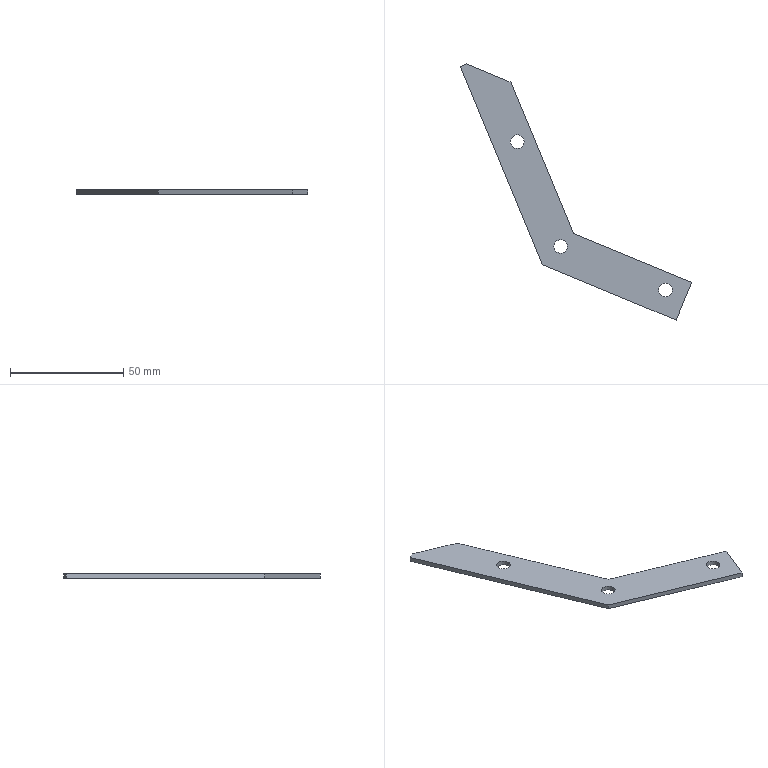Part | SolidWorks | features ICE 6, Cut 1, Extrusion 1, Shell 1 | 1 solid | 15 faces | box 102.016 x 112.94 x 2 mm | volume 5038 mm3 | plane 9 | cylinder 6 | commonest cylinder face diameters 6 x6
STEP:
#1=CARTESIAN_POINT('',(-66.636,-128.964,308.));
#2=VERTEX_POINT('',#1);
#3=CARTESIAN_POINT('',(-60.636,-128.964,308.));
#4=VERTEX_POINT('',#3);
#5=CARTESIAN_POINT('',(-63.636,-128.964,308.));
#6=DIRECTION('',(0.,0.,1.));
#7=DIRECTION('',(1.,0.,0.));
#8=AXIS2_PLACEMENT_3D('',#5,#6,#7);
#9=CIRCLE('',#8,3.);
#10=EDGE_CURVE('',#2,#4,#9,.T.);
#11=ORIENTED_EDGE('',*,*,#10,.F.);
#12=CARTESIAN_POINT('',(-66.636,-128.964,310.));
#13=VERTEX_POINT('',#12);
#14=CARTESIAN_POINT('',(-66.636,-128.964,300.));
#15=DIRECTION('',(0.,0.,1.));
#16=VECTOR('',#15,1000.);
#17=LINE('',#14,#16);
#18=EDGE_CURVE('',#2,#13,#17,.T.);
#19=ORIENTED_EDGE('',*,*,#18,.T.);
#20=CARTESIAN_POINT('',(-60.636,-128.964,310.));
#21=VERTEX_POINT('',#20);
#22=CARTESIAN_POINT('',(-63.636,-128.964,310.));
#23=DIRECTION('',(0.,0.,1.));
#24=DIRECTION('',(-1.,0.,0.));
#25=AXIS2_PLACEMENT_3D('',#22,#23,#24);
#26=CIRCLE('',#25,3.);
#27=EDGE_CURVE('',#13,#21,#26,.T.);
#28=ORIENTED_EDGE('',*,*,#27,.T.);
#29=CARTESIAN_POINT('',(-60.636,-128.964,300.));
#30=DIRECTION('',(0.,0.,1.));
#31=VECTOR('',#30,1000.);
#32=LINE('',#29,#31);
#33=EDGE_CURVE('',#4,#21,#32,.T.);
#34=ORIENTED_EDGE('',*,*,#33,.F.);
#35=EDGE_LOOP('',(#11,#19,#28,#34));
#36=FACE_OUTER_BOUND('',#35,.T.);
#37=CARTESIAN_POINT('',(-63.636,-128.964,300.));
#38=DIRECTION('',(0.,0.,1.));
#39=DIRECTION('',(1.,0.,0.));
#40=AXIS2_PLACEMENT_3D('',#37,#38,#39);
#41=CYLINDRICAL_SURFACE('',#40,3.);
#42=ADVANCED_FACE('',(#36),#41,.F.);
#43=CARTESIAN_POINT('',(-112.83,-109.83,308.));
#44=VERTEX_POINT('',#43);
#45=CARTESIAN_POINT('',(-106.83,-109.83,308.));
#46=VERTEX_POINT('',#45);
#47=CARTESIAN_POINT('',(-109.83,-109.83,308.));
#48=DIRECTION('',(0.,0.,1.));
#49=DIRECTION('',(1.,0.,0.));
#50=AXIS2_PLACEMENT_3D('',#47,#48,#49);
#51=CIRCLE('',#50,3.);
#52=EDGE_CURVE('',#44,#46,#51,.T.);
#53=ORIENTED_EDGE('',*,*,#52,.F.);
#54=CARTESIAN_POINT('',(-112.83,-109.83,310.));
#55=VERTEX_POINT('',#54);
#56=CARTESIAN_POINT('',(-112.83,-109.83,300.));
#57=DIRECTION('',(0.,0.,1.));
#58=VECTOR('',#57,1000.);
#59=LINE('',#56,#58);
#60=EDGE_CURVE('',#44,#55,#59,.T.);
#61=ORIENTED_EDGE('',*,*,#60,.T.);
#62=CARTESIAN_POINT('',(-106.83,-109.83,310.));
#63=VERTEX_POINT('',#62);
#64=CARTESIAN_POINT('',(-109.83,-109.83,310.));
#65=DIRECTION('',(0.,0.,1.));
#66=DIRECTION('',(-1.,0.,0.));
#67=AXIS2_PLACEMENT_3D('',#64,#65,#66);
#68=CIRCLE('',#67,3.);
#69=EDGE_CURVE('',#55,#63,#68,.T.);
#70=ORIENTED_EDGE('',*,*,#69,.T.);
#71=CARTESIAN_POINT('',(-106.83,-109.83,300.));
#72=DIRECTION('',(0.,0.,1.));
#73=VECTOR('',#72,1000.);
#74=LINE('',#71,#73);
#75=EDGE_CURVE('',#46,#63,#74,.T.);
#76=ORIENTED_EDGE('',*,*,#75,.F.);
#77=EDGE_LOOP('',(#53,#61,#70,#76));
#78=FACE_OUTER_BOUND('',#77,.T.);
#79=CARTESIAN_POINT('',(-109.83,-109.83,300.));
#80=DIRECTION('',(0.,0.,1.));
#81=DIRECTION('',(1.,0.,0.));
#82=AXIS2_PLACEMENT_3D('',#79,#80,#81);
#83=CYLINDRICAL_SURFACE('',#82,3.);
#84=ADVANCED_FACE('',(#78),#83,.F.);
#85=CARTESIAN_POINT('',(-131.964,-63.636,308.));
#86=VERTEX_POINT('',#85);
#87=CARTESIAN_POINT('',(-125.964,-63.636,308.));
#88=VERTEX_POINT('',#87);
#89=CARTESIAN_POINT('',(-128.964,-63.636,308.));
#90=DIRECTION('',(0.,0.,1.));
#91=DIRECTION('',(1.,0.,0.));
#92=AXIS2_PLACEMENT_3D('',#89,#90,#91);
#93=CIRCLE('',#92,3.);
#94=EDGE_CURVE('',#86,#88,#93,.T.);
#95=ORIENTED_EDGE('',*,*,#94,.F.);
#96=CARTESIAN_POINT('',(-131.964,-63.636,310.));
#97=VERTEX_POINT('',#96);
#98=CARTESIAN_POINT('',(-131.964,-63.636,300.));
#99=DIRECTION('',(0.,0.,1.));
#100=VECTOR('',#99,1000.);
#101=LINE('',#98,#100);
#102=EDGE_CURVE('',#86,#97,#101,.T.);
#103=ORIENTED_EDGE('',*,*,#102,.T.);
#104=CARTESIAN_POINT('',(-125.964,-63.636,310.));
#105=VERTEX_POINT('',#104);
#106=CARTESIAN_POINT('',(-128.964,-63.636,310.));
#107=DIRECTION('',(0.,0.,1.));
#108=DIRECTION('',(-1.,0.,0.));
#109=AXIS2_PLACEMENT_3D('',#106,#107,#108);
#110=CIRCLE('',#109,3.);
#111=EDGE_CURVE('',#97,#105,#110,.T.);
#112=ORIENTED_EDGE('',*,*,#111,.T.);
#113=CARTESIAN_POINT('',(-125.964,-63.636,300.));
#114=DIRECTION('',(0.,0.,1.));
#115=VECTOR('',#114,1000.);
#116=LINE('',#113,#115);
#117=EDGE_CURVE('',#88,#105,#116,.T.);
#118=ORIENTED_EDGE('',*,*,#117,.F.);
#119=EDGE_LOOP('',(#95,#103,#112,#118));
#120=FACE_OUTER_BOUND('',#119,.T.);
#121=CARTESIAN_POINT('',(-128.964,-63.636,300.));
#122=DIRECTION('',(0.,0.,1.));
#123=DIRECTION('',(1.,0.,0.));
#124=AXIS2_PLACEMENT_3D('',#121,#122,#123);
#125=CYLINDRICAL_SURFACE('',#124,3.);
#126=ADVANCED_FACE('',(#120),#125,.F.);
#127=CARTESIAN_POINT('',(-154.061,-30.485,310.));
#128=VERTEX_POINT('',#127);
#129=CARTESIAN_POINT('',(-151.289,-29.337,310.));
#130=VERTEX_POINT('',#129);
#131=CARTESIAN_POINT('',(-154.061,-30.485,310.));
#132=DIRECTION('',(0.9239,0.3827,0.));
#133=VECTOR('',#132,1000.);
#134=LINE('',#131,#133);
#135=EDGE_CURVE('',#128,#130,#134,.T.);
#136=ORIENTED_EDGE('',*,*,#135,.F.);
#137=CARTESIAN_POINT('',(-117.866,-117.866,310.));
#138=VERTEX_POINT('',#137);
#139=CARTESIAN_POINT('',(-155.209,-27.714,310.));
#140=DIRECTION('',(-0.3827,0.9239,0.));
#141=VECTOR('',#140,1000.);
#142=LINE('',#139,#141);
#143=EDGE_CURVE('',#138,#128,#142,.T.);
#144=ORIENTED_EDGE('',*,*,#143,.F.);
#145=CARTESIAN_POINT('',(-58.933,-142.277,310.));
#146=VERTEX_POINT('',#145);
#147=CARTESIAN_POINT('',(-117.866,-117.866,310.));
#148=DIRECTION('',(-0.9239,0.3827,0.));
#149=VECTOR('',#148,1000.);
#150=LINE('',#147,#149);
#151=EDGE_CURVE('',#146,#138,#150,.T.);
#152=ORIENTED_EDGE('',*,*,#151,.F.);
#153=CARTESIAN_POINT('',(-52.045,-125.648,310.));
#154=VERTEX_POINT('',#153);
#155=CARTESIAN_POINT('',(70.138,169.329,310.));
#156=DIRECTION('',(-0.3827,-0.9239,0.));
#157=VECTOR('',#156,1000.);
#158=LINE('',#155,#157);
#159=EDGE_CURVE('',#154,#146,#158,.T.);
#160=ORIENTED_EDGE('',*,*,#159,.F.);
#161=CARTESIAN_POINT('',(-104.09,-104.09,310.));
#162=VERTEX_POINT('',#161);
#163=CARTESIAN_POINT('',(-104.09,-104.09,310.));
#164=DIRECTION('',(0.9239,-0.3827,0.));
#165=VECTOR('',#164,1000.);
#166=LINE('',#163,#165);
#167=EDGE_CURVE('',#162,#154,#166,.T.);
#168=ORIENTED_EDGE('',*,*,#167,.F.);
#169=CARTESIAN_POINT('',(-131.691,-37.455,310.));
#170=VERTEX_POINT('',#169);
#171=CARTESIAN_POINT('',(-147.205,0.,310.));
#172=DIRECTION('',(0.3827,-0.9239,0.));
#173=VECTOR('',#172,1000.);
#174=LINE('',#171,#173);
#175=EDGE_CURVE('',#170,#162,#174,.T.);
#176=ORIENTED_EDGE('',*,*,#175,.F.);
#177=CARTESIAN_POINT('',(-208.989,-5.437,310.));
#178=DIRECTION('',(0.9239,-0.3827,0.));
#179=VECTOR('',#178,1000.);
#180=LINE('',#177,#179);
#181=EDGE_CURVE('',#130,#170,#180,.T.);
#182=ORIENTED_EDGE('',*,*,#181,.F.);
#183=EDGE_LOOP('',(#136,#144,#152,#160,#168,#176,#182));
#184=FACE_OUTER_BOUND('',#183,.T.);
#185=CARTESIAN_POINT('',(-63.636,-128.964,310.));
#186=DIRECTION('',(0.,0.,1.));
#187=DIRECTION('',(-1.,0.,0.));
#188=AXIS2_PLACEMENT_3D('',#185,#186,#187);
#189=CIRCLE('',#188,3.);
#190=EDGE_CURVE('',#21,#13,#189,.T.);
#191=ORIENTED_EDGE('',*,*,#190,.F.);
#192=ORIENTED_EDGE('',*,*,#27,.F.);
#193=EDGE_LOOP('',(#191,#192));
#194=FACE_BOUND('',#193,.T.);
#195=CARTESIAN_POINT('',(-109.83,-109.83,310.));
#196=DIRECTION('',(0.,0.,1.));
#197=DIRECTION('',(-1.,0.,0.));
#198=AXIS2_PLACEMENT_3D('',#195,#196,#197);
#199=CIRCLE('',#198,3.);
#200=EDGE_CURVE('',#63,#55,#199,.T.);
#201=ORIENTED_EDGE('',*,*,#200,.F.);
#202=ORIENTED_EDGE('',*,*,#69,.F.);
#203=EDGE_LOOP('',(#201,#202));
#204=FACE_BOUND('',#203,.T.);
#205=CARTESIAN_POINT('',(-128.964,-63.636,310.));
#206=DIRECTION('',(0.,0.,1.));
#207=DIRECTION('',(-1.,0.,0.));
#208=AXIS2_PLACEMENT_3D('',#205,#206,#207);
#209=CIRCLE('',#208,3.);
#210=EDGE_CURVE('',#105,#97,#209,.T.);
#211=ORIENTED_EDGE('',*,*,#210,.F.);
#212=ORIENTED_EDGE('',*,*,#111,.F.);
#213=EDGE_LOOP('',(#211,#212));
#214=FACE_BOUND('',#213,.T.);
#215=CARTESIAN_POINT('',(0.,0.,310.));
#216=DIRECTION('',(0.,0.,1.));
#217=DIRECTION('',(1.,0.,0.));
#218=AXIS2_PLACEMENT_3D('',#215,#216,#217);
#219=PLANE('',#218);
#220=ADVANCED_FACE('',(#184,#194,#204,#214),#219,.T.);
#221=CARTESIAN_POINT('',(-63.636,-128.964,308.));
#222=DIRECTION('',(0.,0.,1.));
#223=DIRECTION('',(1.,0.,0.));
#224=AXIS2_PLACEMENT_3D('',#221,#222,#223);
#225=CIRCLE('',#224,3.);
#226=EDGE_CURVE('',#4,#2,#225,.T.);
#227=ORIENTED_EDGE('',*,*,#226,.T.);
#228=ORIENTED_EDGE('',*,*,#10,.T.);
#229=EDGE_LOOP('',(#227,#228));
#230=FACE_BOUND('',#229,.T.);
#231=CARTESIAN_POINT('',(-109.83,-109.83,308.));
#232=DIRECTION('',(0.,0.,1.));
#233=DIRECTION('',(1.,0.,0.));
#234=AXIS2_PLACEMENT_3D('',#231,#232,#233);
#235=CIRCLE('',#234,3.);
#236=EDGE_CURVE('',#46,#44,#235,.T.);
#237=ORIENTED_EDGE('',*,*,#236,.T.);
#238=ORIENTED_EDGE('',*,*,#52,.T.);
#239=EDGE_LOOP('',(#237,#238));
#240=FACE_BOUND('',#239,.T.);
#241=CARTESIAN_POINT('',(-128.964,-63.636,308.));
#242=DIRECTION('',(0.,0.,1.));
#243=DIRECTION('',(1.,0.,0.));
#244=AXIS2_PLACEMENT_3D('',#241,#242,#243);
#245=CIRCLE('',#244,3.);
#246=EDGE_CURVE('',#88,#86,#245,.T.);
#247=ORIENTED_EDGE('',*,*,#246,.T.);
#248=ORIENTED_EDGE('',*,*,#94,.T.);
#249=EDGE_LOOP('',(#247,#248));
#250=FACE_BOUND('',#249,.T.);
#251=CARTESIAN_POINT('',(-117.866,-117.866,308.));
#252=VERTEX_POINT('',#251);
#253=CARTESIAN_POINT('',(-154.061,-30.485,308.));
#254=VERTEX_POINT('',#253);
#255=CARTESIAN_POINT('',(-142.277,-58.933,308.));
#256=DIRECTION('',(-0.3827,0.9239,0.));
#257=VECTOR('',#256,1000.);
#258=LINE('',#255,#257);
#259=EDGE_CURVE('',#252,#254,#258,.T.);
#260=ORIENTED_EDGE('',*,*,#259,.T.);
#261=CARTESIAN_POINT('',(-151.289,-29.337,308.));
#262=VERTEX_POINT('',#261);
#263=CARTESIAN_POINT('',(-154.061,-30.485,308.));
#264=DIRECTION('',(0.9239,0.3827,0.));
#265=VECTOR('',#264,1000.);
#266=LINE('',#263,#265);
#267=EDGE_CURVE('',#254,#262,#266,.T.);
#268=ORIENTED_EDGE('',*,*,#267,.T.);
#269=CARTESIAN_POINT('',(-131.691,-37.455,308.));
#270=VERTEX_POINT('',#269);
#271=CARTESIAN_POINT('',(-32.528,-78.53,308.));
#272=DIRECTION('',(0.9239,-0.3827,0.));
#273=VECTOR('',#272,1000.);
#274=LINE('',#271,#273);
#275=EDGE_CURVE('',#262,#270,#274,.T.);
#276=ORIENTED_EDGE('',*,*,#275,.T.);
#277=CARTESIAN_POINT('',(-104.09,-104.09,308.));
#278=VERTEX_POINT('',#277);
#279=CARTESIAN_POINT('',(-125.648,-52.045,308.));
#280=DIRECTION('',(0.3827,-0.9239,0.));
#281=VECTOR('',#280,1000.);
#282=LINE('',#279,#281);
#283=EDGE_CURVE('',#270,#278,#282,.T.);
#284=ORIENTED_EDGE('',*,*,#283,.T.);
#285=CARTESIAN_POINT('',(-52.045,-125.648,308.));
#286=VERTEX_POINT('',#285);
#287=CARTESIAN_POINT('',(-52.045,-125.648,308.));
#288=DIRECTION('',(0.9239,-0.3827,0.));
#289=VECTOR('',#288,1000.);
#290=LINE('',#287,#289);
#291=EDGE_CURVE('',#278,#286,#290,.T.);
#292=ORIENTED_EDGE('',*,*,#291,.T.);
#293=CARTESIAN_POINT('',(-58.933,-142.277,308.));
#294=VERTEX_POINT('',#293);
#295=CARTESIAN_POINT('',(0.,0.,308.));
#296=DIRECTION('',(-0.3827,-0.9239,0.));
#297=VECTOR('',#296,1000.);
#298=LINE('',#295,#297);
#299=EDGE_CURVE('',#286,#294,#298,.T.);
#300=ORIENTED_EDGE('',*,*,#299,.T.);
#301=CARTESIAN_POINT('',(-58.933,-142.277,308.));
#302=DIRECTION('',(-0.9239,0.3827,0.));
#303=VECTOR('',#302,1000.);
#304=LINE('',#301,#303);
#305=EDGE_CURVE('',#294,#252,#304,.T.);
#306=ORIENTED_EDGE('',*,*,#305,.T.);
#307=EDGE_LOOP('',(#260,#268,#276,#284,#292,#300,#306));
#308=FACE_OUTER_BOUND('',#307,.T.);
#309=CARTESIAN_POINT('',(0.,0.,308.));
#310=DIRECTION('',(0.,0.,1.));
#311=DIRECTION('',(1.,0.,0.));
#312=AXIS2_PLACEMENT_3D('',#309,#310,#311);
#313=PLANE('',#312);
#314=ADVANCED_FACE('',(#230,#240,#250,#308),#313,.F.);
#315=ORIENTED_EDGE('',*,*,#167,.T.);
#316=CARTESIAN_POINT('',(-52.045,-125.648,300.));
#317=DIRECTION('',(0.,0.,-1.));
#318=VECTOR('',#317,1000.);
#319=LINE('',#316,#318);
#320=EDGE_CURVE('',#154,#286,#319,.T.);
#321=ORIENTED_EDGE('',*,*,#320,.T.);
#322=ORIENTED_EDGE('',*,*,#291,.F.);
#323=CARTESIAN_POINT('',(-104.09,-104.09,300.));
#324=DIRECTION('',(0.,0.,1.));
#325=VECTOR('',#324,1000.);
#326=LINE('',#323,#325);
#327=EDGE_CURVE('',#278,#162,#326,.T.);
#328=ORIENTED_EDGE('',*,*,#327,.T.);
#329=EDGE_LOOP('',(#315,#321,#322,#328));
#330=FACE_OUTER_BOUND('',#329,.T.);
#331=CARTESIAN_POINT('',(-104.09,-104.09,300.));
#332=DIRECTION('',(-0.3827,-0.9239,0.));
#333=DIRECTION('',(0.9239,-0.3827,0.));
#334=AXIS2_PLACEMENT_3D('',#331,#332,#333);
#335=PLANE('',#334);
#336=ADVANCED_FACE('',(#330),#335,.F.);
#337=ORIENTED_EDGE('',*,*,#283,.F.);
#338=CARTESIAN_POINT('',(-131.691,-37.455,300.));
#339=DIRECTION('',(0.,0.,1.));
#340=VECTOR('',#339,1000.);
#341=LINE('',#338,#340);
#342=EDGE_CURVE('',#270,#170,#341,.T.);
#343=ORIENTED_EDGE('',*,*,#342,.T.);
#344=ORIENTED_EDGE('',*,*,#175,.T.);
#345=ORIENTED_EDGE('',*,*,#327,.F.);
#346=EDGE_LOOP('',(#337,#343,#344,#345));
#347=FACE_OUTER_BOUND('',#346,.T.);
#348=CARTESIAN_POINT('',(-147.205,0.,300.));
#349=DIRECTION('',(-0.9239,-0.3827,0.));
#350=DIRECTION('',(0.3827,-0.9239,0.));
#351=AXIS2_PLACEMENT_3D('',#348,#349,#350);
#352=PLANE('',#351);
#353=ADVANCED_FACE('',(#347),#352,.F.);
#354=ORIENTED_EDGE('',*,*,#159,.T.);
#355=CARTESIAN_POINT('',(-58.933,-142.277,0.));
#356=DIRECTION('',(0.,0.,-1.));
#357=VECTOR('',#356,1000.);
#358=LINE('',#355,#357);
#359=EDGE_CURVE('',#146,#294,#358,.T.);
#360=ORIENTED_EDGE('',*,*,#359,.T.);
#361=ORIENTED_EDGE('',*,*,#299,.F.);
#362=ORIENTED_EDGE('',*,*,#320,.F.);
#363=EDGE_LOOP('',(#354,#360,#361,#362));
#364=FACE_OUTER_BOUND('',#363,.T.);
#365=CARTESIAN_POINT('',(70.138,169.329,0.));
#366=DIRECTION('',(-0.9239,0.3827,0.));
#367=DIRECTION('',(-0.3827,-0.9239,0.));
#368=AXIS2_PLACEMENT_3D('',#365,#366,#367);
#369=PLANE('',#368);
#370=ADVANCED_FACE('',(#364),#369,.F.);
#371=ORIENTED_EDGE('',*,*,#275,.F.);
#372=CARTESIAN_POINT('',(-151.289,-29.337,308.));
#373=DIRECTION('',(0.,0.,1.));
#374=VECTOR('',#373,1000.);
#375=LINE('',#372,#374);
#376=EDGE_CURVE('',#262,#130,#375,.T.);
#377=ORIENTED_EDGE('',*,*,#376,.T.);
#378=ORIENTED_EDGE('',*,*,#181,.T.);
#379=ORIENTED_EDGE('',*,*,#342,.F.);
#380=EDGE_LOOP('',(#371,#377,#378,#379));
#381=FACE_OUTER_BOUND('',#380,.T.);
#382=CARTESIAN_POINT('',(-208.989,-5.437,305.));
#383=DIRECTION('',(-0.3827,-0.9239,0.));
#384=DIRECTION('',(0.9239,-0.3827,0.));
#385=AXIS2_PLACEMENT_3D('',#382,#383,#384);
#386=PLANE('',#385);
#387=ADVANCED_FACE('',(#381),#386,.F.);
#388=ORIENTED_EDGE('',*,*,#102,.F.);
#389=ORIENTED_EDGE('',*,*,#246,.F.);
#390=ORIENTED_EDGE('',*,*,#117,.T.);
#391=ORIENTED_EDGE('',*,*,#210,.T.);
#392=EDGE_LOOP('',(#388,#389,#390,#391));
#393=FACE_OUTER_BOUND('',#392,.T.);
#394=CARTESIAN_POINT('',(-128.964,-63.636,300.));
#395=DIRECTION('',(0.,0.,1.));
#396=DIRECTION('',(1.,0.,0.));
#397=AXIS2_PLACEMENT_3D('',#394,#395,#396);
#398=CYLINDRICAL_SURFACE('',#397,3.);
#399=ADVANCED_FACE('',(#393),#398,.F.);
#400=ORIENTED_EDGE('',*,*,#60,.F.);
#401=ORIENTED_EDGE('',*,*,#236,.F.);
#402=ORIENTED_EDGE('',*,*,#75,.T.);
#403=ORIENTED_EDGE('',*,*,#200,.T.);
#404=EDGE_LOOP('',(#400,#401,#402,#403));
#405=FACE_OUTER_BOUND('',#404,.T.);
#406=CARTESIAN_POINT('',(-109.83,-109.83,300.));
#407=DIRECTION('',(0.,0.,1.));
#408=DIRECTION('',(1.,0.,0.));
#409=AXIS2_PLACEMENT_3D('',#406,#407,#408);
#410=CYLINDRICAL_SURFACE('',#409,3.);
#411=ADVANCED_FACE('',(#405),#410,.F.);
#412=ORIENTED_EDGE('',*,*,#18,.F.);
#413=ORIENTED_EDGE('',*,*,#226,.F.);
#414=ORIENTED_EDGE('',*,*,#33,.T.);
#415=ORIENTED_EDGE('',*,*,#190,.T.);
#416=EDGE_LOOP('',(#412,#413,#414,#415));
#417=FACE_OUTER_BOUND('',#416,.T.);
#418=CARTESIAN_POINT('',(-63.636,-128.964,300.));
#419=DIRECTION('',(0.,0.,1.));
#420=DIRECTION('',(1.,0.,0.));
#421=AXIS2_PLACEMENT_3D('',#418,#419,#420);
#422=CYLINDRICAL_SURFACE('',#421,3.);
#423=ADVANCED_FACE('',(#417),#422,.F.);
#424=ORIENTED_EDGE('',*,*,#359,.F.);
#425=ORIENTED_EDGE('',*,*,#151,.T.);
#426=CARTESIAN_POINT('',(-117.866,-117.866,0.));
#427=DIRECTION('',(0.,0.,1.));
#428=VECTOR('',#427,1000.);
#429=LINE('',#426,#428);
#430=EDGE_CURVE('',#252,#138,#429,.T.);
#431=ORIENTED_EDGE('',*,*,#430,.F.);
#432=ORIENTED_EDGE('',*,*,#305,.F.);
#433=EDGE_LOOP('',(#424,#425,#431,#432));
#434=FACE_OUTER_BOUND('',#433,.T.);
#435=CARTESIAN_POINT('',(-117.866,-117.866,0.));
#436=DIRECTION('',(0.3827,0.9239,0.));
#437=DIRECTION('',(-0.9239,0.3827,0.));
#438=AXIS2_PLACEMENT_3D('',#435,#436,#437);
#439=PLANE('',#438);
#440=ADVANCED_FACE('',(#434),#439,.F.);
#441=ORIENTED_EDGE('',*,*,#143,.T.);
#442=CARTESIAN_POINT('',(-154.061,-30.485,308.));
#443=DIRECTION('',(0.,0.,1.));
#444=VECTOR('',#443,1000.);
#445=LINE('',#442,#444);
#446=EDGE_CURVE('',#254,#128,#445,.T.);
#447=ORIENTED_EDGE('',*,*,#446,.F.);
#448=ORIENTED_EDGE('',*,*,#259,.F.);
#449=ORIENTED_EDGE('',*,*,#430,.T.);
#450=EDGE_LOOP('',(#441,#447,#448,#449));
#451=FACE_OUTER_BOUND('',#450,.T.);
#452=CARTESIAN_POINT('',(-155.209,-27.714,0.));
#453=DIRECTION('',(0.9239,0.3827,0.));
#454=DIRECTION('',(-0.3827,0.9239,0.));
#455=AXIS2_PLACEMENT_3D('',#452,#453,#454);
#456=PLANE('',#455);
#457=ADVANCED_FACE('',(#451),#456,.F.);
#458=ORIENTED_EDGE('',*,*,#135,.T.);
#459=ORIENTED_EDGE('',*,*,#376,.F.);
#460=ORIENTED_EDGE('',*,*,#267,.F.);
#461=ORIENTED_EDGE('',*,*,#446,.T.);
#462=EDGE_LOOP('',(#458,#459,#460,#461));
#463=FACE_OUTER_BOUND('',#462,.T.);
#464=CARTESIAN_POINT('',(-154.061,-30.485,308.));
#465=DIRECTION('',(0.3827,-0.9239,0.));
#466=DIRECTION('',(0.9239,0.3827,0.));
#467=AXIS2_PLACEMENT_3D('',#464,#465,#466);
#468=PLANE('',#467);
#469=ADVANCED_FACE('',(#463),#468,.F.);
#470=CLOSED_SHELL('',(#42,#84,#126,#220,#314,#336,#353,#370,#387,#399,#411,#423,#440,#457,#469));
#471=MANIFOLD_SOLID_BREP('',#470);
#472=CARTESIAN_POINT('',(0.,0.,0.));
#473=DIRECTION('',(0.,0.,1.));
#474=DIRECTION('',(1.,0.,0.));
#475=AXIS2_PLACEMENT_3D('',#472,#473,#474);
#476=(LENGTH_UNIT()NAMED_UNIT(*)SI_UNIT(.MILLI.,.METRE.));
#477=UNCERTAINTY_MEASURE_WITH_UNIT(LENGTH_MEASURE(0.00001),#476,'','');
#478=(NAMED_UNIT(*)PLANE_ANGLE_UNIT()SI_UNIT($,.RADIAN.));
#479=(NAMED_UNIT(*)SI_UNIT($,.STERADIAN.)SOLID_ANGLE_UNIT());
#480=(GEOMETRIC_REPRESENTATION_CONTEXT(3)GLOBAL_UNCERTAINTY_ASSIGNED_CONTEXT((#477))GLOBAL_UNIT_ASSIGNED_CONTEXT((#476,#478,#479))REPRESENTATION_CONTEXT('',''));
#481=ADVANCED_BREP_SHAPE_REPRESENTATION('',(#471,#475),#480);